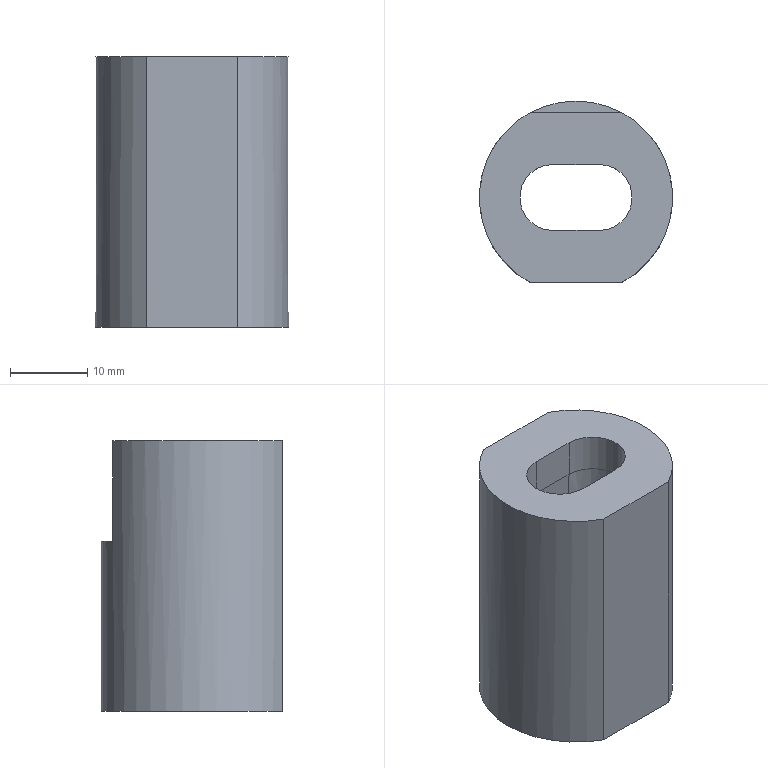Part | STEP file | lll_id4522_x_t | 1 solid | 14 faces | box 25 x 23.5 x 35 mm | volume 12321 mm3 | plane 9 | cylinder 3 | cone 2 | commonest cylinder face diameters 8.55 x2 25 x1
STEP:
#1=CARTESIAN_POINT('',(3593.171,-241.45,0.00001673));
#2=VERTEX_POINT('',#1);
#3=CARTESIAN_POINT('',(3581.297,-241.45,0.00001673));
#4=VERTEX_POINT('',#3);
#5=CARTESIAN_POINT('',(3587.234,-241.45,0.00001673));
#6=DIRECTION('',(-1.,0.,0.));
#7=VECTOR('',#6,1.);
#8=LINE('',#5,#7);
#9=EDGE_CURVE('',#2,#4,#8,.T.);
#10=ORIENTED_EDGE('',*,*,#9,.F.);
#11=CARTESIAN_POINT('',(3593.171,-219.45,0.00001673));
#12=VERTEX_POINT('',#11);
#13=CARTESIAN_POINT('',(3587.234,-230.45,0.00001673));
#14=DIRECTION('',(0.,0.,-1.));
#15=DIRECTION('',(-1.,0.,0.));
#16=AXIS2_PLACEMENT_3D('',#13,#14,#15);
#17=CIRCLE('',#16,12.5);
#18=EDGE_CURVE('',#12,#2,#17,.T.);
#19=ORIENTED_EDGE('',*,*,#18,.F.);
#20=CARTESIAN_POINT('',(3581.297,-219.45,0.00001673));
#21=VERTEX_POINT('',#20);
#22=CARTESIAN_POINT('',(3587.234,-219.45,0.00001673));
#23=DIRECTION('',(-1.,0.,0.));
#24=VECTOR('',#23,1.);
#25=LINE('',#22,#24);
#26=EDGE_CURVE('',#12,#21,#25,.T.);
#27=ORIENTED_EDGE('',*,*,#26,.T.);
#28=CARTESIAN_POINT('',(3587.234,-230.45,0.00001673));
#29=DIRECTION('',(0.,0.,-1.));
#30=DIRECTION('',(-1.,0.,0.));
#31=AXIS2_PLACEMENT_3D('',#28,#29,#30);
#32=CIRCLE('',#31,12.5);
#33=EDGE_CURVE('',#4,#21,#32,.T.);
#34=ORIENTED_EDGE('',*,*,#33,.F.);
#35=EDGE_LOOP('',(#10,#19,#27,#34));
#36=FACE_BOUND('',#35,.T.);
#37=CARTESIAN_POINT('',(3584.234,-226.175,0.00001673));
#38=VERTEX_POINT('',#37);
#39=CARTESIAN_POINT('',(3590.234,-226.175,0.00001673));
#40=VERTEX_POINT('',#39);
#41=CARTESIAN_POINT('',(3587.234,-226.175,0.00001673));
#42=DIRECTION('',(1.,0.,0.));
#43=VECTOR('',#42,1.);
#44=LINE('',#41,#43);
#45=EDGE_CURVE('',#38,#40,#44,.T.);
#46=ORIENTED_EDGE('',*,*,#45,.T.);
#47=CARTESIAN_POINT('',(3590.234,-234.725,0.00001673));
#48=VERTEX_POINT('',#47);
#49=CARTESIAN_POINT('',(3590.234,-230.45,0.00001673));
#50=DIRECTION('',(0.,0.,-1.));
#51=DIRECTION('',(-1.,0.,0.));
#52=AXIS2_PLACEMENT_3D('',#49,#50,#51);
#53=CIRCLE('',#52,4.275);
#54=EDGE_CURVE('',#40,#48,#53,.T.);
#55=ORIENTED_EDGE('',*,*,#54,.T.);
#56=CARTESIAN_POINT('',(3584.234,-234.725,0.00001673));
#57=VERTEX_POINT('',#56);
#58=CARTESIAN_POINT('',(3587.234,-234.725,0.00001673));
#59=DIRECTION('',(-1.,0.,0.));
#60=VECTOR('',#59,1.);
#61=LINE('',#58,#60);
#62=EDGE_CURVE('',#48,#57,#61,.T.);
#63=ORIENTED_EDGE('',*,*,#62,.T.);
#64=CARTESIAN_POINT('',(3584.234,-230.45,0.00001673));
#65=DIRECTION('',(0.,0.,-1.));
#66=DIRECTION('',(-1.,0.,0.));
#67=AXIS2_PLACEMENT_3D('',#64,#65,#66);
#68=CIRCLE('',#67,4.275);
#69=EDGE_CURVE('',#57,#38,#68,.T.);
#70=ORIENTED_EDGE('',*,*,#69,.T.);
#71=EDGE_LOOP('',(#46,#55,#63,#70));
#72=FACE_BOUND('',#71,.T.);
#73=CARTESIAN_POINT('',(3587.234,-230.45,0.00001673));
#74=DIRECTION('',(0.,0.,1.));
#75=DIRECTION('',(1.,0.,0.));
#76=AXIS2_PLACEMENT_3D('',#73,#74,#75);
#77=PLANE('',#76);
#78=ADVANCED_FACE('',(#36,#72),#77,.T.);
#79=CARTESIAN_POINT('',(3593.171,-241.45,-35.));
#80=VERTEX_POINT('',#79);
#81=CARTESIAN_POINT('',(3593.171,-241.45,-15.));
#82=DIRECTION('',(0.,0.,-1.));
#83=VECTOR('',#82,1.);
#84=LINE('',#81,#83);
#85=EDGE_CURVE('',#2,#80,#84,.T.);
#86=ORIENTED_EDGE('',*,*,#85,.T.);
#87=CARTESIAN_POINT('',(3581.297,-241.45,-35.));
#88=VERTEX_POINT('',#87);
#89=CARTESIAN_POINT('',(3587.234,-230.45,-35.));
#90=DIRECTION('',(0.,0.,-1.));
#91=DIRECTION('',(-1.,0.,0.));
#92=AXIS2_PLACEMENT_3D('',#89,#90,#91);
#93=CIRCLE('',#92,12.5);
#94=EDGE_CURVE('',#88,#80,#93,.T.);
#95=ORIENTED_EDGE('',*,*,#94,.F.);
#96=CARTESIAN_POINT('',(3581.297,-241.45,-15.));
#97=DIRECTION('',(0.,0.,1.));
#98=VECTOR('',#97,1.);
#99=LINE('',#96,#98);
#100=EDGE_CURVE('',#88,#4,#99,.T.);
#101=ORIENTED_EDGE('',*,*,#100,.T.);
#102=ORIENTED_EDGE('',*,*,#33,.T.);
#103=CARTESIAN_POINT('',(3581.297,-219.45,-13.));
#104=VERTEX_POINT('',#103);
#105=CARTESIAN_POINT('',(3581.297,-219.45,-15.));
#106=DIRECTION('',(0.,0.,-1.));
#107=VECTOR('',#106,1.);
#108=LINE('',#105,#107);
#109=EDGE_CURVE('',#21,#104,#108,.T.);
#110=ORIENTED_EDGE('',*,*,#109,.T.);
#111=CARTESIAN_POINT('',(3593.171,-219.45,-13.));
#112=VERTEX_POINT('',#111);
#113=CARTESIAN_POINT('',(3587.234,-230.45,-13.));
#114=DIRECTION('',(0.,0.,1.));
#115=DIRECTION('',(-1.,0.,0.));
#116=AXIS2_PLACEMENT_3D('',#113,#114,#115);
#117=CIRCLE('',#116,12.5);
#118=EDGE_CURVE('',#112,#104,#117,.T.);
#119=ORIENTED_EDGE('',*,*,#118,.F.);
#120=CARTESIAN_POINT('',(3593.171,-219.45,-15.));
#121=DIRECTION('',(0.,0.,1.));
#122=VECTOR('',#121,1.);
#123=LINE('',#120,#122);
#124=EDGE_CURVE('',#112,#12,#123,.T.);
#125=ORIENTED_EDGE('',*,*,#124,.T.);
#126=ORIENTED_EDGE('',*,*,#18,.T.);
#127=EDGE_LOOP('',(#86,#95,#101,#102,#110,#119,#125,#126));
#128=FACE_OUTER_BOUND('',#127,.T.);
#129=CARTESIAN_POINT('',(3587.234,-230.45,-15.));
#130=DIRECTION('',(0.,0.,-1.));
#131=DIRECTION('',(0.,-1.,0.));
#132=AXIS2_PLACEMENT_3D('',#129,#130,#131);
#133=CYLINDRICAL_SURFACE('',#132,12.5);
#134=ADVANCED_FACE('',(#128),#133,.T.);
#135=CARTESIAN_POINT('',(3587.234,-241.45,-35.));
#136=DIRECTION('',(-1.,0.,0.));
#137=VECTOR('',#136,1.);
#138=LINE('',#135,#137);
#139=EDGE_CURVE('',#80,#88,#138,.T.);
#140=ORIENTED_EDGE('',*,*,#139,.T.);
#141=ORIENTED_EDGE('',*,*,#94,.T.);
#142=EDGE_LOOP('',(#140,#141));
#143=FACE_BOUND('',#142,.T.);
#144=CARTESIAN_POINT('',(3584.234,-235.511,-35.));
#145=VERTEX_POINT('',#144);
#146=CARTESIAN_POINT('',(3590.234,-235.511,-35.));
#147=VERTEX_POINT('',#146);
#148=CARTESIAN_POINT('',(3587.234,-235.511,-35.));
#149=DIRECTION('',(1.,0.,0.));
#150=VECTOR('',#149,1.);
#151=LINE('',#148,#150);
#152=EDGE_CURVE('',#145,#147,#151,.T.);
#153=ORIENTED_EDGE('',*,*,#152,.T.);
#154=CARTESIAN_POINT('',(3590.234,-225.389,-35.));
#155=VERTEX_POINT('',#154);
#156=CARTESIAN_POINT('',(3590.234,-230.45,-35.));
#157=DIRECTION('',(0.,0.,1.));
#158=DIRECTION('',(-1.,0.,0.));
#159=AXIS2_PLACEMENT_3D('',#156,#157,#158);
#160=CIRCLE('',#159,5.061);
#161=EDGE_CURVE('',#147,#155,#160,.T.);
#162=ORIENTED_EDGE('',*,*,#161,.T.);
#163=CARTESIAN_POINT('',(3584.234,-225.389,-35.));
#164=VERTEX_POINT('',#163);
#165=CARTESIAN_POINT('',(3587.234,-225.389,-35.));
#166=DIRECTION('',(-1.,0.,0.));
#167=VECTOR('',#166,1.);
#168=LINE('',#165,#167);
#169=EDGE_CURVE('',#155,#164,#168,.T.);
#170=ORIENTED_EDGE('',*,*,#169,.T.);
#171=CARTESIAN_POINT('',(3584.234,-230.45,-35.));
#172=DIRECTION('',(0.,0.,1.));
#173=DIRECTION('',(-1.,0.,0.));
#174=AXIS2_PLACEMENT_3D('',#171,#172,#173);
#175=CIRCLE('',#174,5.061);
#176=EDGE_CURVE('',#164,#145,#175,.T.);
#177=ORIENTED_EDGE('',*,*,#176,.T.);
#178=EDGE_LOOP('',(#153,#162,#170,#177));
#179=FACE_BOUND('',#178,.T.);
#180=CARTESIAN_POINT('',(3587.234,-235.95,-35.));
#181=DIRECTION('',(0.,0.,-1.));
#182=DIRECTION('',(0.,1.,0.));
#183=AXIS2_PLACEMENT_3D('',#180,#181,#182);
#184=PLANE('',#183);
#185=ADVANCED_FACE('',(#143,#179),#184,.T.);
#186=CARTESIAN_POINT('',(3590.234,-226.175,-5.));
#187=VERTEX_POINT('',#186);
#188=CARTESIAN_POINT('',(3590.234,-226.175,2.5));
#189=DIRECTION('',(-0.000000008,0.,1.));
#190=VECTOR('',#189,1.);
#191=LINE('',#188,#190);
#192=EDGE_CURVE('',#187,#40,#191,.T.);
#193=ORIENTED_EDGE('',*,*,#192,.F.);
#194=CARTESIAN_POINT('',(3590.234,-234.725,-5.));
#195=VERTEX_POINT('',#194);
#196=CARTESIAN_POINT('',(3590.234,-230.45,-5.));
#197=DIRECTION('',(0.,0.,-1.));
#198=DIRECTION('',(-1.,0.,0.));
#199=AXIS2_PLACEMENT_3D('',#196,#197,#198);
#200=CIRCLE('',#199,4.275);
#201=EDGE_CURVE('',#187,#195,#200,.T.);
#202=ORIENTED_EDGE('',*,*,#201,.T.);
#203=CARTESIAN_POINT('',(3590.234,-234.725,2.5));
#204=DIRECTION('',(-0.000000008,0.,1.));
#205=VECTOR('',#204,1.);
#206=LINE('',#203,#205);
#207=EDGE_CURVE('',#195,#48,#206,.T.);
#208=ORIENTED_EDGE('',*,*,#207,.T.);
#209=ORIENTED_EDGE('',*,*,#54,.F.);
#210=EDGE_LOOP('',(#193,#202,#208,#209));
#211=FACE_OUTER_BOUND('',#210,.T.);
#212=CARTESIAN_POINT('',(3590.234,-230.45,2.5));
#213=DIRECTION('',(-0.000000008,0.,1.));
#214=DIRECTION('',(-1.,0.,-0.000000008));
#215=AXIS2_PLACEMENT_3D('',#212,#213,#214);
#216=CYLINDRICAL_SURFACE('',#215,4.275);
#217=ADVANCED_FACE('',(#211),#216,.F.);
#218=CARTESIAN_POINT('',(3584.234,-226.175,-5.));
#219=VERTEX_POINT('',#218);
#220=CARTESIAN_POINT('',(3584.234,-226.175,2.5));
#221=DIRECTION('',(-0.000000008,0.,1.));
#222=VECTOR('',#221,1.);
#223=LINE('',#220,#222);
#224=EDGE_CURVE('',#219,#38,#223,.T.);
#225=ORIENTED_EDGE('',*,*,#224,.F.);
#226=CARTESIAN_POINT('',(3584.234,-226.175,-5.));
#227=DIRECTION('',(1.,0.,0.));
#228=VECTOR('',#227,1.);
#229=LINE('',#226,#228);
#230=EDGE_CURVE('',#219,#187,#229,.T.);
#231=ORIENTED_EDGE('',*,*,#230,.T.);
#232=ORIENTED_EDGE('',*,*,#192,.T.);
#233=ORIENTED_EDGE('',*,*,#45,.F.);
#234=EDGE_LOOP('',(#225,#231,#232,#233));
#235=FACE_OUTER_BOUND('',#234,.T.);
#236=CARTESIAN_POINT('',(3584.234,-226.175,2.5));
#237=DIRECTION('',(0.,-1.,0.));
#238=DIRECTION('',(1.,0.,0.000000008));
#239=AXIS2_PLACEMENT_3D('',#236,#237,#238);
#240=PLANE('',#239);
#241=ADVANCED_FACE('',(#235),#240,.T.);
#242=CARTESIAN_POINT('',(3584.234,-234.725,-5.));
#243=VERTEX_POINT('',#242);
#244=CARTESIAN_POINT('',(3584.234,-234.725,2.5));
#245=DIRECTION('',(-0.000000008,0.,1.));
#246=VECTOR('',#245,1.);
#247=LINE('',#244,#246);
#248=EDGE_CURVE('',#243,#57,#247,.T.);
#249=ORIENTED_EDGE('',*,*,#248,.F.);
#250=CARTESIAN_POINT('',(3584.234,-230.45,-5.));
#251=DIRECTION('',(0.,0.,-1.));
#252=DIRECTION('',(-1.,0.,0.));
#253=AXIS2_PLACEMENT_3D('',#250,#251,#252);
#254=CIRCLE('',#253,4.275);
#255=EDGE_CURVE('',#243,#219,#254,.T.);
#256=ORIENTED_EDGE('',*,*,#255,.T.);
#257=ORIENTED_EDGE('',*,*,#224,.T.);
#258=ORIENTED_EDGE('',*,*,#69,.F.);
#259=EDGE_LOOP('',(#249,#256,#257,#258));
#260=FACE_OUTER_BOUND('',#259,.T.);
#261=CARTESIAN_POINT('',(3584.234,-230.45,2.5));
#262=DIRECTION('',(-0.000000008,0.,1.));
#263=DIRECTION('',(-1.,0.,-0.000000008));
#264=AXIS2_PLACEMENT_3D('',#261,#262,#263);
#265=CYLINDRICAL_SURFACE('',#264,4.275);
#266=ADVANCED_FACE('',(#260),#265,.F.);
#267=ORIENTED_EDGE('',*,*,#207,.F.);
#268=CARTESIAN_POINT('',(3590.234,-234.725,-5.));
#269=DIRECTION('',(-1.,0.,0.));
#270=VECTOR('',#269,1.);
#271=LINE('',#268,#270);
#272=EDGE_CURVE('',#195,#243,#271,.T.);
#273=ORIENTED_EDGE('',*,*,#272,.T.);
#274=ORIENTED_EDGE('',*,*,#248,.T.);
#275=ORIENTED_EDGE('',*,*,#62,.F.);
#276=EDGE_LOOP('',(#267,#273,#274,#275));
#277=FACE_OUTER_BOUND('',#276,.T.);
#278=CARTESIAN_POINT('',(3584.234,-234.725,2.5));
#279=DIRECTION('',(0.,-1.,0.));
#280=DIRECTION('',(1.,0.,0.000000008));
#281=AXIS2_PLACEMENT_3D('',#278,#279,#280);
#282=PLANE('',#281);
#283=ADVANCED_FACE('',(#277),#282,.F.);
#284=CARTESIAN_POINT('',(3590.234,-234.725,-5.));
#285=DIRECTION('',(0.,-0.02618,-0.9997));
#286=VECTOR('',#285,1.);
#287=LINE('',#284,#286);
#288=EDGE_CURVE('',#195,#147,#287,.T.);
#289=ORIENTED_EDGE('',*,*,#288,.F.);
#290=ORIENTED_EDGE('',*,*,#201,.F.);
#291=CARTESIAN_POINT('',(3590.234,-226.175,-5.));
#292=DIRECTION('',(0.,0.02618,-0.9997));
#293=VECTOR('',#292,1.);
#294=LINE('',#291,#293);
#295=EDGE_CURVE('',#187,#155,#294,.T.);
#296=ORIENTED_EDGE('',*,*,#295,.T.);
#297=ORIENTED_EDGE('',*,*,#161,.F.);
#298=EDGE_LOOP('',(#289,#290,#296,#297));
#299=FACE_OUTER_BOUND('',#298,.T.);
#300=CARTESIAN_POINT('',(3590.234,-230.45,-5.));
#301=DIRECTION('',(0.,0.,-1.));
#302=DIRECTION('',(-1.,0.,0.));
#303=AXIS2_PLACEMENT_3D('',#300,#301,#302);
#304=CONICAL_SURFACE('',#303,4.275,1.5);
#305=ADVANCED_FACE('',(#299),#304,.F.);
#306=CARTESIAN_POINT('',(3584.234,-234.725,-5.));
#307=DIRECTION('',(-0.000000001,-0.02618,-0.9997));
#308=VECTOR('',#307,1.);
#309=LINE('',#306,#308);
#310=EDGE_CURVE('',#243,#145,#309,.T.);
#311=ORIENTED_EDGE('',*,*,#310,.F.);
#312=ORIENTED_EDGE('',*,*,#272,.F.);
#313=ORIENTED_EDGE('',*,*,#288,.T.);
#314=ORIENTED_EDGE('',*,*,#152,.F.);
#315=EDGE_LOOP('',(#311,#312,#313,#314));
#316=FACE_OUTER_BOUND('',#315,.T.);
#317=CARTESIAN_POINT('',(3590.234,-234.725,-5.));
#318=DIRECTION('',(0.,0.9997,-0.02618));
#319=DIRECTION('',(0.,0.02618,0.9997));
#320=AXIS2_PLACEMENT_3D('',#317,#318,#319);
#321=PLANE('',#320);
#322=ADVANCED_FACE('',(#316),#321,.T.);
#323=CARTESIAN_POINT('',(3584.234,-226.175,-5.));
#324=DIRECTION('',(0.,0.02618,-0.9997));
#325=VECTOR('',#324,1.);
#326=LINE('',#323,#325);
#327=EDGE_CURVE('',#219,#164,#326,.T.);
#328=ORIENTED_EDGE('',*,*,#327,.F.);
#329=ORIENTED_EDGE('',*,*,#255,.F.);
#330=ORIENTED_EDGE('',*,*,#310,.T.);
#331=ORIENTED_EDGE('',*,*,#176,.F.);
#332=EDGE_LOOP('',(#328,#329,#330,#331));
#333=FACE_OUTER_BOUND('',#332,.T.);
#334=CARTESIAN_POINT('',(3584.234,-230.45,-5.));
#335=DIRECTION('',(0.,0.,-1.));
#336=DIRECTION('',(-1.,0.,0.));
#337=AXIS2_PLACEMENT_3D('',#334,#335,#336);
#338=CONICAL_SURFACE('',#337,4.275,1.5);
#339=ADVANCED_FACE('',(#333),#338,.F.);
#340=ORIENTED_EDGE('',*,*,#295,.F.);
#341=ORIENTED_EDGE('',*,*,#230,.F.);
#342=ORIENTED_EDGE('',*,*,#327,.T.);
#343=ORIENTED_EDGE('',*,*,#169,.F.);
#344=EDGE_LOOP('',(#340,#341,#342,#343));
#345=FACE_OUTER_BOUND('',#344,.T.);
#346=CARTESIAN_POINT('',(3584.234,-226.175,-5.));
#347=DIRECTION('',(0.,-0.9997,-0.02618));
#348=DIRECTION('',(0.,0.02618,-0.9997));
#349=AXIS2_PLACEMENT_3D('',#346,#347,#348);
#350=PLANE('',#349);
#351=ADVANCED_FACE('',(#345),#350,.T.);
#352=ORIENTED_EDGE('',*,*,#26,.F.);
#353=ORIENTED_EDGE('',*,*,#124,.F.);
#354=CARTESIAN_POINT('',(3595.234,-219.45,-13.));
#355=DIRECTION('',(-1.,0.,0.));
#356=VECTOR('',#355,1.);
#357=LINE('',#354,#356);
#358=EDGE_CURVE('',#112,#104,#357,.T.);
#359=ORIENTED_EDGE('',*,*,#358,.T.);
#360=ORIENTED_EDGE('',*,*,#109,.F.);
#361=EDGE_LOOP('',(#352,#353,#359,#360));
#362=FACE_OUTER_BOUND('',#361,.T.);
#363=CARTESIAN_POINT('',(3568.842,-219.45,-17.5));
#364=DIRECTION('',(0.,-1.,0.));
#365=DIRECTION('',(0.,0.,-1.));
#366=AXIS2_PLACEMENT_3D('',#363,#364,#365);
#367=PLANE('',#366);
#368=ADVANCED_FACE('',(#362),#367,.F.);
#369=ORIENTED_EDGE('',*,*,#118,.T.);
#370=ORIENTED_EDGE('',*,*,#358,.F.);
#371=EDGE_LOOP('',(#369,#370));
#372=FACE_OUTER_BOUND('',#371,.T.);
#373=CARTESIAN_POINT('',(3595.234,-211.45,-13.));
#374=DIRECTION('',(0.,0.,-1.));
#375=DIRECTION('',(-1.,0.,0.));
#376=AXIS2_PLACEMENT_3D('',#373,#374,#375);
#377=PLANE('',#376);
#378=ADVANCED_FACE('',(#372),#377,.F.);
#379=ORIENTED_EDGE('',*,*,#9,.T.);
#380=ORIENTED_EDGE('',*,*,#100,.F.);
#381=ORIENTED_EDGE('',*,*,#139,.F.);
#382=ORIENTED_EDGE('',*,*,#85,.F.);
#383=EDGE_LOOP('',(#379,#380,#381,#382));
#384=FACE_OUTER_BOUND('',#383,.T.);
#385=CARTESIAN_POINT('',(3587.234,-241.45,-6.5));
#386=DIRECTION('',(0.,1.,0.));
#387=DIRECTION('',(0.,0.,1.));
#388=AXIS2_PLACEMENT_3D('',#385,#386,#387);
#389=PLANE('',#388);
#390=ADVANCED_FACE('',(#384),#389,.F.);
#391=CLOSED_SHELL('',(#78,#134,#185,#217,#241,#266,#283,#305,#322,#339,#351,#368,#378,#390));
#392=MANIFOLD_SOLID_BREP('',#391);
#393=(LENGTH_UNIT()NAMED_UNIT(*)SI_UNIT(.MILLI.,.METRE.));
#394=UNCERTAINTY_MEASURE_WITH_UNIT(LENGTH_MEASURE(0.00002),#393,'','');
#395=(NAMED_UNIT(*)PLANE_ANGLE_UNIT()SI_UNIT($,.RADIAN.));
#396=PLANE_ANGLE_MEASURE_WITH_UNIT(PLANE_ANGLE_MEASURE(0.01745),#395);
#397=DIMENSIONAL_EXPONENTS(0.,0.,0.,0.,0.,0.,0.);
#398=(CONVERSION_BASED_UNIT('DEGREE',#396)NAMED_UNIT(#397)PLANE_ANGLE_UNIT());
#399=(NAMED_UNIT(*)SI_UNIT($,.STERADIAN.)SOLID_ANGLE_UNIT());
#400=(GEOMETRIC_REPRESENTATION_CONTEXT(3)GLOBAL_UNCERTAINTY_ASSIGNED_CONTEXT((#394))GLOBAL_UNIT_ASSIGNED_CONTEXT((#393,#398,#399))REPRESENTATION_CONTEXT('',''));
#401=ADVANCED_BREP_SHAPE_REPRESENTATION('',(#392),#400);